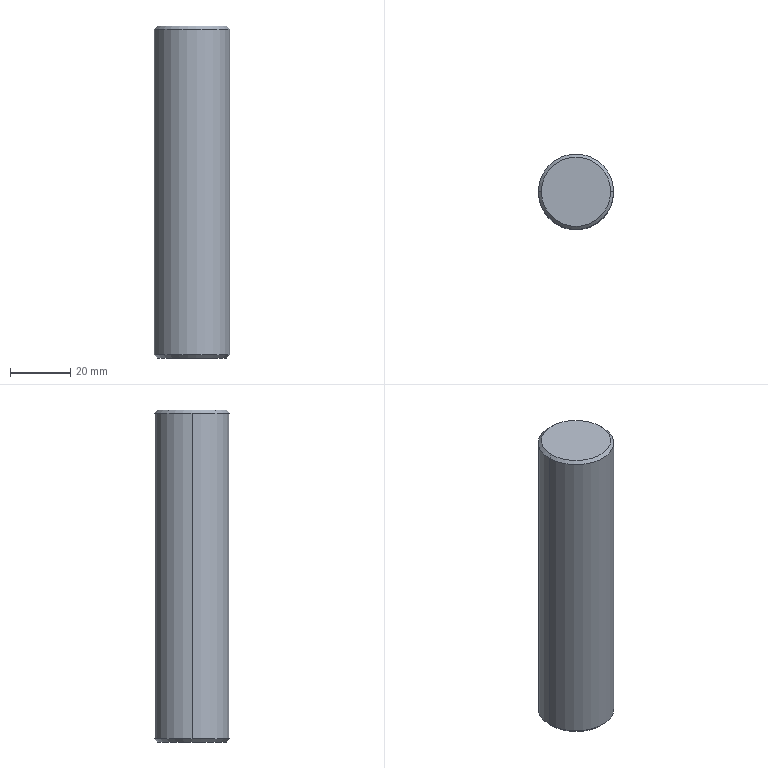Part | SolidWorks | features BaseBody 1 | 1 solid | 12 faces | box 25 x 25 x 110 mm | volume 53576 mm3 | cone 6 | cylinder 4 | plane 2 | commonest cylinder face diameters 5 x2 25 x2
STEP:
#1=CARTESIAN_POINT('',(2.5,0.,-38.));
#2=VERTEX_POINT('',#1);
#3=CARTESIAN_POINT('',(-2.5,0.,-38.));
#4=VERTEX_POINT('',#3);
#5=CARTESIAN_POINT('',(0.,0.,-38.));
#6=DIRECTION('',(0.,0.,-1.));
#7=DIRECTION('',(-1.,0.,0.));
#8=AXIS2_PLACEMENT_3D('',#5,#6,#7);
#9=CIRCLE('',#8,2.5);
#10=EDGE_CURVE('',#2,#4,#9,.T.);
#11=ORIENTED_EDGE('',*,*,#10,.F.);
#12=CARTESIAN_POINT('',(2.5,0.,-55.));
#13=VERTEX_POINT('',#12);
#14=CARTESIAN_POINT('',(2.5,0.,-55.));
#15=DIRECTION('',(0.,0.,-1.));
#16=VECTOR('',#15,1000.);
#17=LINE('',#14,#16);
#18=EDGE_CURVE('',#2,#13,#17,.T.);
#19=ORIENTED_EDGE('',*,*,#18,.T.);
#20=CARTESIAN_POINT('',(-2.5,0.,-55.));
#21=VERTEX_POINT('',#20);
#22=CARTESIAN_POINT('',(0.,0.,-55.));
#23=DIRECTION('',(0.,0.,-1.));
#24=DIRECTION('',(-1.,0.,0.));
#25=AXIS2_PLACEMENT_3D('',#22,#23,#24);
#26=CIRCLE('',#25,2.5);
#27=EDGE_CURVE('',#13,#21,#26,.T.);
#28=ORIENTED_EDGE('',*,*,#27,.T.);
#29=CARTESIAN_POINT('',(-2.5,0.,-55.));
#30=DIRECTION('',(0.,0.,-1.));
#31=VECTOR('',#30,1000.);
#32=LINE('',#29,#31);
#33=EDGE_CURVE('',#4,#21,#32,.T.);
#34=ORIENTED_EDGE('',*,*,#33,.F.);
#35=EDGE_LOOP('',(#11,#19,#28,#34));
#36=FACE_OUTER_BOUND('',#35,.T.);
#37=CARTESIAN_POINT('',(0.,0.,-55.));
#38=DIRECTION('',(0.,0.,-1.));
#39=DIRECTION('',(-1.,0.,0.));
#40=AXIS2_PLACEMENT_3D('',#37,#38,#39);
#41=CYLINDRICAL_SURFACE('',#40,2.5);
#42=ADVANCED_FACE('',(#36),#41,.F.);
#43=CARTESIAN_POINT('',(0.,0.,-36.498));
#44=VERTEX_POINT('',#43);
#45=CARTESIAN_POINT('',(-2.5,0.,-38.));
#46=DIRECTION('',(-0.8572,0.,-0.515));
#47=VECTOR('',#46,1000.);
#48=LINE('',#45,#47);
#49=EDGE_CURVE('',#44,#4,#48,.T.);
#50=ORIENTED_EDGE('',*,*,#49,.F.);
#51=CARTESIAN_POINT('',(2.5,0.,-38.));
#52=DIRECTION('',(0.8572,0.,-0.515));
#53=VECTOR('',#52,1000.);
#54=LINE('',#51,#53);
#55=EDGE_CURVE('',#44,#2,#54,.T.);
#56=ORIENTED_EDGE('',*,*,#55,.T.);
#57=ORIENTED_EDGE('',*,*,#10,.T.);
#58=EDGE_LOOP('',(#50,#56,#57));
#59=FACE_OUTER_BOUND('',#58,.T.);
#60=CARTESIAN_POINT('',(0.,0.,-38.));
#61=DIRECTION('',(0.,0.,-1.));
#62=DIRECTION('',(-1.,0.,0.));
#63=AXIS2_PLACEMENT_3D('',#60,#61,#62);
#64=CONICAL_SURFACE('',#63,2.5,1.03);
#65=ADVANCED_FACE('',(#59),#64,.F.);
#66=CARTESIAN_POINT('',(-11.5,0.,-55.));
#67=VERTEX_POINT('',#66);
#68=CARTESIAN_POINT('',(11.5,0.,-55.));
#69=VERTEX_POINT('',#68);
#70=CARTESIAN_POINT('',(0.,0.,-55.));
#71=DIRECTION('',(0.,0.,-1.));
#72=DIRECTION('',(1.,0.,0.));
#73=AXIS2_PLACEMENT_3D('',#70,#71,#72);
#74=CIRCLE('',#73,11.5);
#75=EDGE_CURVE('',#67,#69,#74,.T.);
#76=ORIENTED_EDGE('',*,*,#75,.F.);
#77=CARTESIAN_POINT('',(-12.5,0.,-54.));
#78=VERTEX_POINT('',#77);
#79=CARTESIAN_POINT('',(-12.5,0.,-54.));
#80=DIRECTION('',(-0.7071,0.,0.7071));
#81=VECTOR('',#80,1000.);
#82=LINE('',#79,#81);
#83=EDGE_CURVE('',#67,#78,#82,.T.);
#84=ORIENTED_EDGE('',*,*,#83,.T.);
#85=CARTESIAN_POINT('',(12.5,0.,-54.));
#86=VERTEX_POINT('',#85);
#87=CARTESIAN_POINT('',(0.,0.,-54.));
#88=DIRECTION('',(0.,0.,1.));
#89=DIRECTION('',(1.,0.,0.));
#90=AXIS2_PLACEMENT_3D('',#87,#88,#89);
#91=CIRCLE('',#90,12.5);
#92=EDGE_CURVE('',#86,#78,#91,.T.);
#93=ORIENTED_EDGE('',*,*,#92,.F.);
#94=CARTESIAN_POINT('',(12.5,0.,-54.));
#95=DIRECTION('',(0.7071,0.,0.7071));
#96=VECTOR('',#95,1000.);
#97=LINE('',#94,#96);
#98=EDGE_CURVE('',#69,#86,#97,.T.);
#99=ORIENTED_EDGE('',*,*,#98,.F.);
#100=EDGE_LOOP('',(#76,#84,#93,#99));
#101=FACE_OUTER_BOUND('',#100,.T.);
#102=CARTESIAN_POINT('',(0.,0.,-54.));
#103=DIRECTION('',(0.,0.,1.));
#104=DIRECTION('',(1.,0.,0.));
#105=AXIS2_PLACEMENT_3D('',#102,#103,#104);
#106=CONICAL_SURFACE('',#105,12.5,0.7854);
#107=ADVANCED_FACE('',(#101),#106,.T.);
#108=CARTESIAN_POINT('',(11.5,0.,55.));
#109=VERTEX_POINT('',#108);
#110=CARTESIAN_POINT('',(-11.5,0.,55.));
#111=VERTEX_POINT('',#110);
#112=CARTESIAN_POINT('',(0.,0.,55.));
#113=DIRECTION('',(0.,0.,1.));
#114=DIRECTION('',(1.,0.,0.));
#115=AXIS2_PLACEMENT_3D('',#112,#113,#114);
#116=CIRCLE('',#115,11.5);
#117=EDGE_CURVE('',#109,#111,#116,.T.);
#118=ORIENTED_EDGE('',*,*,#117,.F.);
#119=CARTESIAN_POINT('',(12.5,0.,54.));
#120=VERTEX_POINT('',#119);
#121=CARTESIAN_POINT('',(11.5,0.,55.));
#122=DIRECTION('',(0.7071,0.,-0.7071));
#123=VECTOR('',#122,1000.);
#124=LINE('',#121,#123);
#125=EDGE_CURVE('',#109,#120,#124,.T.);
#126=ORIENTED_EDGE('',*,*,#125,.T.);
#127=CARTESIAN_POINT('',(-12.5,0.,54.));
#128=VERTEX_POINT('',#127);
#129=CARTESIAN_POINT('',(0.,0.,54.));
#130=DIRECTION('',(0.,0.,-1.));
#131=DIRECTION('',(1.,0.,0.));
#132=AXIS2_PLACEMENT_3D('',#129,#130,#131);
#133=CIRCLE('',#132,12.5);
#134=EDGE_CURVE('',#128,#120,#133,.T.);
#135=ORIENTED_EDGE('',*,*,#134,.F.);
#136=CARTESIAN_POINT('',(-11.5,0.,55.));
#137=DIRECTION('',(-0.7071,0.,-0.7071));
#138=VECTOR('',#137,1000.);
#139=LINE('',#136,#138);
#140=EDGE_CURVE('',#111,#128,#139,.T.);
#141=ORIENTED_EDGE('',*,*,#140,.F.);
#142=EDGE_LOOP('',(#118,#126,#135,#141));
#143=FACE_OUTER_BOUND('',#142,.T.);
#144=CARTESIAN_POINT('',(0.,0.,55.));
#145=DIRECTION('',(0.,0.,-1.));
#146=DIRECTION('',(-1.,0.,0.));
#147=AXIS2_PLACEMENT_3D('',#144,#145,#146);
#148=CONICAL_SURFACE('',#147,11.5,0.7854);
#149=ADVANCED_FACE('',(#143),#148,.T.);
#150=ORIENTED_EDGE('',*,*,#134,.T.);
#151=CARTESIAN_POINT('',(12.5,0.,55.));
#152=DIRECTION('',(0.,0.,-1.));
#153=VECTOR('',#152,1000.);
#154=LINE('',#151,#153);
#155=EDGE_CURVE('',#120,#86,#154,.T.);
#156=ORIENTED_EDGE('',*,*,#155,.T.);
#157=ORIENTED_EDGE('',*,*,#92,.T.);
#158=CARTESIAN_POINT('',(-12.5,0.,55.));
#159=DIRECTION('',(0.,0.,-1.));
#160=VECTOR('',#159,1000.);
#161=LINE('',#158,#160);
#162=EDGE_CURVE('',#128,#78,#161,.T.);
#163=ORIENTED_EDGE('',*,*,#162,.F.);
#164=EDGE_LOOP('',(#150,#156,#157,#163));
#165=FACE_OUTER_BOUND('',#164,.T.);
#166=CARTESIAN_POINT('',(0.,0.,55.));
#167=DIRECTION('',(0.,0.,-1.));
#168=DIRECTION('',(-1.,0.,0.));
#169=AXIS2_PLACEMENT_3D('',#166,#167,#168);
#170=CYLINDRICAL_SURFACE('',#169,12.5);
#171=ADVANCED_FACE('',(#165),#170,.T.);
#172=ORIENTED_EDGE('',*,*,#155,.F.);
#173=CARTESIAN_POINT('',(0.,0.,54.));
#174=DIRECTION('',(0.,0.,-1.));
#175=DIRECTION('',(1.,0.,0.));
#176=AXIS2_PLACEMENT_3D('',#173,#174,#175);
#177=CIRCLE('',#176,12.5);
#178=EDGE_CURVE('',#120,#128,#177,.T.);
#179=ORIENTED_EDGE('',*,*,#178,.T.);
#180=ORIENTED_EDGE('',*,*,#162,.T.);
#181=CARTESIAN_POINT('',(0.,0.,-54.));
#182=DIRECTION('',(0.,0.,1.));
#183=DIRECTION('',(1.,0.,0.));
#184=AXIS2_PLACEMENT_3D('',#181,#182,#183);
#185=CIRCLE('',#184,12.5);
#186=EDGE_CURVE('',#78,#86,#185,.T.);
#187=ORIENTED_EDGE('',*,*,#186,.T.);
#188=EDGE_LOOP('',(#172,#179,#180,#187));
#189=FACE_OUTER_BOUND('',#188,.T.);
#190=CARTESIAN_POINT('',(0.,0.,55.));
#191=DIRECTION('',(0.,0.,-1.));
#192=DIRECTION('',(-1.,0.,0.));
#193=AXIS2_PLACEMENT_3D('',#190,#191,#192);
#194=CYLINDRICAL_SURFACE('',#193,12.5);
#195=ADVANCED_FACE('',(#189),#194,.T.);
#196=CARTESIAN_POINT('',(0.,0.,55.));
#197=DIRECTION('',(0.,0.,1.));
#198=DIRECTION('',(1.,0.,0.));
#199=AXIS2_PLACEMENT_3D('',#196,#197,#198);
#200=CIRCLE('',#199,11.5);
#201=EDGE_CURVE('',#111,#109,#200,.T.);
#202=ORIENTED_EDGE('',*,*,#201,.T.);
#203=ORIENTED_EDGE('',*,*,#117,.T.);
#204=EDGE_LOOP('',(#202,#203));
#205=FACE_OUTER_BOUND('',#204,.T.);
#206=CARTESIAN_POINT('',(0.,0.,55.));
#207=DIRECTION('',(0.,0.,1.));
#208=DIRECTION('',(1.,0.,0.));
#209=AXIS2_PLACEMENT_3D('',#206,#207,#208);
#210=PLANE('',#209);
#211=ADVANCED_FACE('',(#205),#210,.T.);
#212=CARTESIAN_POINT('',(0.,0.,-55.));
#213=DIRECTION('',(0.,0.,-1.));
#214=DIRECTION('',(-1.,0.,0.));
#215=AXIS2_PLACEMENT_3D('',#212,#213,#214);
#216=CIRCLE('',#215,2.5);
#217=EDGE_CURVE('',#21,#13,#216,.T.);
#218=ORIENTED_EDGE('',*,*,#217,.F.);
#219=ORIENTED_EDGE('',*,*,#27,.F.);
#220=EDGE_LOOP('',(#218,#219));
#221=FACE_BOUND('',#220,.T.);
#222=CARTESIAN_POINT('',(0.,0.,-55.));
#223=DIRECTION('',(0.,0.,-1.));
#224=DIRECTION('',(1.,0.,0.));
#225=AXIS2_PLACEMENT_3D('',#222,#223,#224);
#226=CIRCLE('',#225,11.5);
#227=EDGE_CURVE('',#69,#67,#226,.T.);
#228=ORIENTED_EDGE('',*,*,#227,.T.);
#229=ORIENTED_EDGE('',*,*,#75,.T.);
#230=EDGE_LOOP('',(#228,#229));
#231=FACE_OUTER_BOUND('',#230,.T.);
#232=CARTESIAN_POINT('',(0.,0.,-55.));
#233=DIRECTION('',(0.,0.,1.));
#234=DIRECTION('',(1.,0.,0.));
#235=AXIS2_PLACEMENT_3D('',#232,#233,#234);
#236=PLANE('',#235);
#237=ADVANCED_FACE('',(#221,#231),#236,.F.);
#238=ORIENTED_EDGE('',*,*,#125,.F.);
#239=ORIENTED_EDGE('',*,*,#201,.F.);
#240=ORIENTED_EDGE('',*,*,#140,.T.);
#241=ORIENTED_EDGE('',*,*,#178,.F.);
#242=EDGE_LOOP('',(#238,#239,#240,#241));
#243=FACE_OUTER_BOUND('',#242,.T.);
#244=CARTESIAN_POINT('',(0.,0.,55.));
#245=DIRECTION('',(0.,0.,-1.));
#246=DIRECTION('',(-1.,0.,0.));
#247=AXIS2_PLACEMENT_3D('',#244,#245,#246);
#248=CONICAL_SURFACE('',#247,11.5,0.7854);
#249=ADVANCED_FACE('',(#243),#248,.T.);
#250=ORIENTED_EDGE('',*,*,#83,.F.);
#251=ORIENTED_EDGE('',*,*,#227,.F.);
#252=ORIENTED_EDGE('',*,*,#98,.T.);
#253=ORIENTED_EDGE('',*,*,#186,.F.);
#254=EDGE_LOOP('',(#250,#251,#252,#253));
#255=FACE_OUTER_BOUND('',#254,.T.);
#256=CARTESIAN_POINT('',(0.,0.,-54.));
#257=DIRECTION('',(0.,0.,1.));
#258=DIRECTION('',(1.,0.,0.));
#259=AXIS2_PLACEMENT_3D('',#256,#257,#258);
#260=CONICAL_SURFACE('',#259,12.5,0.7854);
#261=ADVANCED_FACE('',(#255),#260,.T.);
#262=ORIENTED_EDGE('',*,*,#55,.F.);
#263=ORIENTED_EDGE('',*,*,#49,.T.);
#264=CARTESIAN_POINT('',(0.,0.,-38.));
#265=DIRECTION('',(0.,0.,-1.));
#266=DIRECTION('',(-1.,0.,0.));
#267=AXIS2_PLACEMENT_3D('',#264,#265,#266);
#268=CIRCLE('',#267,2.5);
#269=EDGE_CURVE('',#4,#2,#268,.T.);
#270=ORIENTED_EDGE('',*,*,#269,.T.);
#271=EDGE_LOOP('',(#262,#263,#270));
#272=FACE_OUTER_BOUND('',#271,.T.);
#273=CARTESIAN_POINT('',(0.,0.,-38.));
#274=DIRECTION('',(0.,0.,-1.));
#275=DIRECTION('',(-1.,0.,0.));
#276=AXIS2_PLACEMENT_3D('',#273,#274,#275);
#277=CONICAL_SURFACE('',#276,2.5,1.03);
#278=ADVANCED_FACE('',(#272),#277,.F.);
#279=ORIENTED_EDGE('',*,*,#18,.F.);
#280=ORIENTED_EDGE('',*,*,#269,.F.);
#281=ORIENTED_EDGE('',*,*,#33,.T.);
#282=ORIENTED_EDGE('',*,*,#217,.T.);
#283=EDGE_LOOP('',(#279,#280,#281,#282));
#284=FACE_OUTER_BOUND('',#283,.T.);
#285=CARTESIAN_POINT('',(0.,0.,-55.));
#286=DIRECTION('',(0.,0.,-1.));
#287=DIRECTION('',(-1.,0.,0.));
#288=AXIS2_PLACEMENT_3D('',#285,#286,#287);
#289=CYLINDRICAL_SURFACE('',#288,2.5);
#290=ADVANCED_FACE('',(#284),#289,.F.);
#291=CLOSED_SHELL('',(#42,#65,#107,#149,#171,#195,#211,#237,#249,#261,#278,#290));
#292=MANIFOLD_SOLID_BREP('',#291);
#293=CARTESIAN_POINT('',(0.,0.,0.));
#294=DIRECTION('',(0.,0.,1.));
#295=DIRECTION('',(1.,0.,0.));
#296=AXIS2_PLACEMENT_3D('',#293,#294,#295);
#297=(LENGTH_UNIT()NAMED_UNIT(*)SI_UNIT(.MILLI.,.METRE.));
#298=UNCERTAINTY_MEASURE_WITH_UNIT(LENGTH_MEASURE(0.00001),#297,'','');
#299=(NAMED_UNIT(*)PLANE_ANGLE_UNIT()SI_UNIT($,.RADIAN.));
#300=(NAMED_UNIT(*)SI_UNIT($,.STERADIAN.)SOLID_ANGLE_UNIT());
#301=(GEOMETRIC_REPRESENTATION_CONTEXT(3)GLOBAL_UNCERTAINTY_ASSIGNED_CONTEXT((#298))GLOBAL_UNIT_ASSIGNED_CONTEXT((#297,#299,#300))REPRESENTATION_CONTEXT('',''));
#302=ADVANCED_BREP_SHAPE_REPRESENTATION('',(#292,#296),#301);